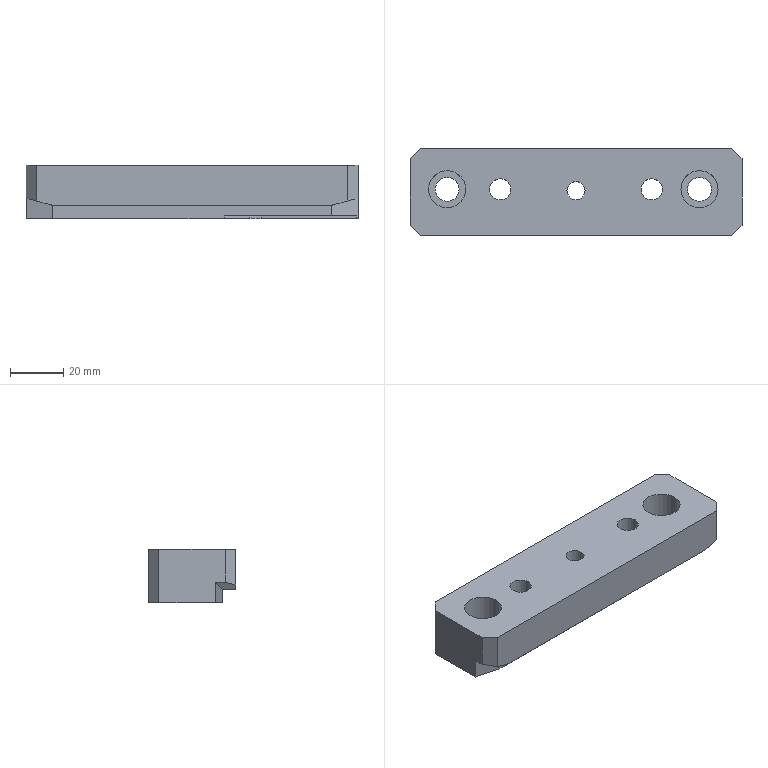Part | NX | features 20 2 | 1 solid | 30 faces | box 125 x 33 x 20 mm | volume 71217 mm3 | plane 21 | cylinder 9 | commonest cylinder face diameters 8.001 x2 9 x2 14 x2 20 x2 6.8 x1
STEP:
#1=CARTESIAN_POINT('',(1124.402,434.5,-3.5));
#2=VERTEX_POINT('',#1);
#3=CARTESIAN_POINT('',(1121.002,434.5,-3.5));
#4=DIRECTION('',(0.,0.,1.));
#5=DIRECTION('',(1.,0.,0.));
#6=AXIS2_PLACEMENT_3D('',#3,#4,#5);
#7=CIRCLE('',#6,3.4);
#8=EDGE_CURVE('',#2,#2,#7,.T.);
#9=ORIENTED_EDGE('',*,*,#8,.T.);
#10=EDGE_LOOP('',(#9));
#11=FACE_BOUND('',#10,.T.);
#12=CARTESIAN_POINT('',(1068.501,422.5,-3.5));
#13=VERTEX_POINT('',#12);
#14=CARTESIAN_POINT('',(1058.502,425.179,-3.5));
#15=VERTEX_POINT('',#14);
#16=CARTESIAN_POINT('',(1068.501,422.5,-3.5));
#17=DIRECTION('',(-0.9659,0.2588,0.));
#18=VECTOR('',#17,1000.);
#19=LINE('',#16,#18);
#20=EDGE_CURVE('',#13,#15,#19,.T.);
#21=ORIENTED_EDGE('',*,*,#20,.T.);
#22=CARTESIAN_POINT('',(1058.502,446.5,-3.5));
#23=VERTEX_POINT('',#22);
#24=CARTESIAN_POINT('',(1058.502,417.5,-3.5));
#25=DIRECTION('',(0.,1.,0.));
#26=VECTOR('',#25,1000.);
#27=LINE('',#24,#26);
#28=EDGE_CURVE('',#15,#23,#27,.T.);
#29=ORIENTED_EDGE('',*,*,#28,.T.);
#30=CARTESIAN_POINT('',(1062.502,450.5,-3.5));
#31=VERTEX_POINT('',#30);
#32=CARTESIAN_POINT('',(1062.502,450.5,-3.5));
#33=DIRECTION('',(-0.7071,-0.7071,0.));
#34=VECTOR('',#33,1000.);
#35=LINE('',#32,#34);
#36=EDGE_CURVE('',#31,#23,#35,.T.);
#37=ORIENTED_EDGE('',*,*,#36,.F.);
#38=CARTESIAN_POINT('',(1179.502,450.5,-3.5));
#39=VERTEX_POINT('',#38);
#40=CARTESIAN_POINT('',(1176.502,450.5,-3.5));
#41=DIRECTION('',(1.,0.,0.));
#42=VECTOR('',#41,1000.);
#43=LINE('',#40,#42);
#44=EDGE_CURVE('',#31,#39,#43,.T.);
#45=ORIENTED_EDGE('',*,*,#44,.T.);
#46=CARTESIAN_POINT('',(1183.502,446.5,-3.5));
#47=VERTEX_POINT('',#46);
#48=CARTESIAN_POINT('',(1183.502,446.5,-3.5));
#49=DIRECTION('',(-0.7071,0.7071,0.));
#50=VECTOR('',#49,1000.);
#51=LINE('',#48,#50);
#52=EDGE_CURVE('',#47,#39,#51,.T.);
#53=ORIENTED_EDGE('',*,*,#52,.F.);
#54=CARTESIAN_POINT('',(1183.502,427.984,-3.5));
#55=VERTEX_POINT('',#54);
#56=CARTESIAN_POINT('',(1183.502,450.5,-3.5));
#57=DIRECTION('',(0.,-1.,0.));
#58=VECTOR('',#57,1000.);
#59=LINE('',#56,#58);
#60=EDGE_CURVE('',#47,#55,#59,.T.);
#61=ORIENTED_EDGE('',*,*,#60,.T.);
#62=CARTESIAN_POINT('',(1182.929,428.,-3.5));
#63=VERTEX_POINT('',#62);
#64=CARTESIAN_POINT('',(1182.929,418.,-3.5));
#65=DIRECTION('',(0.,0.,-1.));
#66=DIRECTION('',(1.,0.,0.));
#67=AXIS2_PLACEMENT_3D('',#64,#65,#66);
#68=CIRCLE('',#67,10.);
#69=EDGE_CURVE('',#63,#55,#68,.T.);
#70=ORIENTED_EDGE('',*,*,#69,.F.);
#71=CARTESIAN_POINT('',(1147.07,428.,-3.5));
#72=VERTEX_POINT('',#71);
#73=CARTESIAN_POINT('',(1066.502,428.,-3.5));
#74=DIRECTION('',(-1.,0.,0.));
#75=VECTOR('',#74,1000.);
#76=LINE('',#73,#75);
#77=EDGE_CURVE('',#63,#72,#76,.T.);
#78=ORIENTED_EDGE('',*,*,#77,.T.);
#79=CARTESIAN_POINT('',(1142.83,427.057,-3.5));
#80=VERTEX_POINT('',#79);
#81=CARTESIAN_POINT('',(1147.07,418.,-3.5));
#82=DIRECTION('',(0.,0.,1.));
#83=DIRECTION('',(1.,0.,0.));
#84=AXIS2_PLACEMENT_3D('',#81,#82,#83);
#85=CIRCLE('',#84,10.);
#86=EDGE_CURVE('',#72,#80,#85,.T.);
#87=ORIENTED_EDGE('',*,*,#86,.T.);
#88=CARTESIAN_POINT('',(1133.095,422.5,-3.5));
#89=VERTEX_POINT('',#88);
#90=CARTESIAN_POINT('',(1089.222,401.964,-3.5));
#91=DIRECTION('',(0.9057,0.4239,0.));
#92=VECTOR('',#91,1000.);
#93=LINE('',#90,#92);
#94=EDGE_CURVE('',#89,#80,#93,.T.);
#95=ORIENTED_EDGE('',*,*,#94,.F.);
#96=CARTESIAN_POINT('',(1154.501,422.5,-3.5));
#97=DIRECTION('',(-1.,0.,0.));
#98=VECTOR('',#97,1000.);
#99=LINE('',#96,#98);
#100=EDGE_CURVE('',#89,#13,#99,.T.);
#101=ORIENTED_EDGE('',*,*,#100,.T.);
#102=EDGE_LOOP('',(#21,#29,#37,#45,#53,#61,#70,#78,#87,#95,#101));
#103=FACE_BOUND('',#102,.T.);
#104=CARTESIAN_POINT('',(1077.002,435.,-3.5));
#105=VERTEX_POINT('',#104);
#106=CARTESIAN_POINT('',(1072.502,435.,-3.5));
#107=DIRECTION('',(0.,0.,1.));
#108=DIRECTION('',(1.,0.,0.));
#109=AXIS2_PLACEMENT_3D('',#106,#107,#108);
#110=CIRCLE('',#109,4.5);
#111=EDGE_CURVE('',#105,#105,#110,.T.);
#112=ORIENTED_EDGE('',*,*,#111,.T.);
#113=EDGE_LOOP('',(#112));
#114=FACE_BOUND('',#113,.T.);
#115=CARTESIAN_POINT('',(1172.002,435.,-3.5));
#116=VERTEX_POINT('',#115);
#117=CARTESIAN_POINT('',(1167.502,435.,-3.5));
#118=DIRECTION('',(0.,0.,-1.));
#119=DIRECTION('',(1.,0.,0.));
#120=AXIS2_PLACEMENT_3D('',#117,#118,#119);
#121=CIRCLE('',#120,4.5);
#122=EDGE_CURVE('',#116,#116,#121,.T.);
#123=ORIENTED_EDGE('',*,*,#122,.F.);
#124=EDGE_LOOP('',(#123));
#125=FACE_BOUND('',#124,.T.);
#126=CARTESIAN_POINT('',(1096.503,435.,-3.5));
#127=VERTEX_POINT('',#126);
#128=CARTESIAN_POINT('',(1092.502,435.,-3.5));
#129=DIRECTION('',(0.,0.,1.));
#130=DIRECTION('',(1.,0.,0.));
#131=AXIS2_PLACEMENT_3D('',#128,#129,#130);
#132=CIRCLE('',#131,4.);
#133=EDGE_CURVE('',#127,#127,#132,.T.);
#134=ORIENTED_EDGE('',*,*,#133,.T.);
#135=EDGE_LOOP('',(#134));
#136=FACE_BOUND('',#135,.T.);
#137=CARTESIAN_POINT('',(1153.503,435.,-3.5));
#138=VERTEX_POINT('',#137);
#139=CARTESIAN_POINT('',(1149.502,435.,-3.5));
#140=DIRECTION('',(0.,0.,-1.));
#141=DIRECTION('',(1.,0.,0.));
#142=AXIS2_PLACEMENT_3D('',#139,#140,#141);
#143=CIRCLE('',#142,4.);
#144=EDGE_CURVE('',#138,#138,#143,.T.);
#145=ORIENTED_EDGE('',*,*,#144,.F.);
#146=EDGE_LOOP('',(#145));
#147=FACE_BOUND('',#146,.T.);
#148=CARTESIAN_POINT('',(1246.502,450.5,-3.5));
#149=DIRECTION('',(0.,0.,1.));
#150=DIRECTION('',(-1.,0.,0.));
#151=AXIS2_PLACEMENT_3D('',#148,#149,#150);
#152=PLANE('',#151);
#153=ADVANCED_FACE('',(#11,#103,#114,#125,#136,#147),#152,.F.);
#154=CARTESIAN_POINT('',(1153.503,435.,16.5));
#155=VERTEX_POINT('',#154);
#156=CARTESIAN_POINT('',(1149.502,435.,16.5));
#157=DIRECTION('',(0.,0.,1.));
#158=DIRECTION('',(1.,0.,0.));
#159=AXIS2_PLACEMENT_3D('',#156,#157,#158);
#160=CIRCLE('',#159,4.);
#161=EDGE_CURVE('',#155,#155,#160,.T.);
#162=ORIENTED_EDGE('',*,*,#161,.F.);
#163=EDGE_LOOP('',(#162));
#164=FACE_BOUND('',#163,.T.);
#165=CARTESIAN_POINT('',(1096.503,435.,16.5));
#166=VERTEX_POINT('',#165);
#167=CARTESIAN_POINT('',(1092.502,435.,16.5));
#168=DIRECTION('',(0.,0.,1.));
#169=DIRECTION('',(1.,0.,0.));
#170=AXIS2_PLACEMENT_3D('',#167,#168,#169);
#171=CIRCLE('',#170,4.);
#172=EDGE_CURVE('',#166,#166,#171,.T.);
#173=ORIENTED_EDGE('',*,*,#172,.F.);
#174=EDGE_LOOP('',(#173));
#175=FACE_BOUND('',#174,.T.);
#176=CARTESIAN_POINT('',(1079.502,435.,16.5));
#177=VERTEX_POINT('',#176);
#178=CARTESIAN_POINT('',(1072.502,435.,16.5));
#179=DIRECTION('',(0.,0.,-1.));
#180=DIRECTION('',(1.,0.,0.));
#181=AXIS2_PLACEMENT_3D('',#178,#179,#180);
#182=CIRCLE('',#181,7.);
#183=EDGE_CURVE('',#177,#177,#182,.T.);
#184=ORIENTED_EDGE('',*,*,#183,.T.);
#185=EDGE_LOOP('',(#184));
#186=FACE_BOUND('',#185,.T.);
#187=CARTESIAN_POINT('',(1183.502,446.5,16.5));
#188=VERTEX_POINT('',#187);
#189=CARTESIAN_POINT('',(1183.502,421.5,16.5));
#190=VERTEX_POINT('',#189);
#191=CARTESIAN_POINT('',(1183.502,450.5,16.5));
#192=DIRECTION('',(0.,-1.,0.));
#193=VECTOR('',#192,1000.);
#194=LINE('',#191,#193);
#195=EDGE_CURVE('',#188,#190,#194,.T.);
#196=ORIENTED_EDGE('',*,*,#195,.F.);
#197=CARTESIAN_POINT('',(1179.502,450.5,16.5));
#198=VERTEX_POINT('',#197);
#199=CARTESIAN_POINT('',(1183.502,446.5,16.5));
#200=DIRECTION('',(0.7071,-0.7071,0.));
#201=VECTOR('',#200,1000.);
#202=LINE('',#199,#201);
#203=EDGE_CURVE('',#198,#188,#202,.T.);
#204=ORIENTED_EDGE('',*,*,#203,.F.);
#205=CARTESIAN_POINT('',(1062.502,450.5,16.5));
#206=VERTEX_POINT('',#205);
#207=CARTESIAN_POINT('',(1136.502,450.5,16.5));
#208=DIRECTION('',(1.,0.,0.));
#209=VECTOR('',#208,1000.);
#210=LINE('',#207,#209);
#211=EDGE_CURVE('',#206,#198,#210,.T.);
#212=ORIENTED_EDGE('',*,*,#211,.F.);
#213=CARTESIAN_POINT('',(1058.502,446.5,16.5));
#214=VERTEX_POINT('',#213);
#215=CARTESIAN_POINT('',(1062.502,450.5,16.5));
#216=DIRECTION('',(0.7071,0.7071,0.));
#217=VECTOR('',#216,1000.);
#218=LINE('',#215,#217);
#219=EDGE_CURVE('',#214,#206,#218,.T.);
#220=ORIENTED_EDGE('',*,*,#219,.F.);
#221=CARTESIAN_POINT('',(1058.502,421.5,16.5));
#222=VERTEX_POINT('',#221);
#223=CARTESIAN_POINT('',(1058.502,417.5,16.5));
#224=DIRECTION('',(0.,1.,0.));
#225=VECTOR('',#224,1000.);
#226=LINE('',#223,#225);
#227=EDGE_CURVE('',#222,#214,#226,.T.);
#228=ORIENTED_EDGE('',*,*,#227,.F.);
#229=CARTESIAN_POINT('',(1062.502,417.5,16.5));
#230=VERTEX_POINT('',#229);
#231=CARTESIAN_POINT('',(1058.502,421.5,16.5));
#232=DIRECTION('',(-0.7071,0.7071,0.));
#233=VECTOR('',#232,1000.);
#234=LINE('',#231,#233);
#235=EDGE_CURVE('',#230,#222,#234,.T.);
#236=ORIENTED_EDGE('',*,*,#235,.F.);
#237=CARTESIAN_POINT('',(1179.502,417.5,16.5));
#238=VERTEX_POINT('',#237);
#239=CARTESIAN_POINT('',(1216.502,417.5,16.5));
#240=DIRECTION('',(-1.,0.,0.));
#241=VECTOR('',#240,1000.);
#242=LINE('',#239,#241);
#243=EDGE_CURVE('',#238,#230,#242,.T.);
#244=ORIENTED_EDGE('',*,*,#243,.F.);
#245=CARTESIAN_POINT('',(1179.502,417.5,16.5));
#246=DIRECTION('',(-0.7071,-0.7071,0.));
#247=VECTOR('',#246,1000.);
#248=LINE('',#245,#247);
#249=EDGE_CURVE('',#190,#238,#248,.T.);
#250=ORIENTED_EDGE('',*,*,#249,.F.);
#251=EDGE_LOOP('',(#196,#204,#212,#220,#228,#236,#244,#250));
#252=FACE_BOUND('',#251,.T.);
#253=CARTESIAN_POINT('',(1174.502,435.,16.5));
#254=VERTEX_POINT('',#253);
#255=CARTESIAN_POINT('',(1167.502,435.,16.5));
#256=DIRECTION('',(0.,0.,-1.));
#257=DIRECTION('',(1.,0.,0.));
#258=AXIS2_PLACEMENT_3D('',#255,#256,#257);
#259=CIRCLE('',#258,7.);
#260=EDGE_CURVE('',#254,#254,#259,.T.);
#261=ORIENTED_EDGE('',*,*,#260,.T.);
#262=EDGE_LOOP('',(#261));
#263=FACE_BOUND('',#262,.T.);
#264=CARTESIAN_POINT('',(1124.402,434.5,16.5));
#265=VERTEX_POINT('',#264);
#266=CARTESIAN_POINT('',(1121.002,434.5,16.5));
#267=DIRECTION('',(0.,0.,1.));
#268=DIRECTION('',(1.,0.,0.));
#269=AXIS2_PLACEMENT_3D('',#266,#267,#268);
#270=CIRCLE('',#269,3.4);
#271=EDGE_CURVE('',#265,#265,#270,.T.);
#272=ORIENTED_EDGE('',*,*,#271,.F.);
#273=EDGE_LOOP('',(#272));
#274=FACE_BOUND('',#273,.T.);
#275=CARTESIAN_POINT('',(1216.502,450.5,16.5));
#276=DIRECTION('',(0.,0.,1.));
#277=DIRECTION('',(-1.,0.,0.));
#278=AXIS2_PLACEMENT_3D('',#275,#276,#277);
#279=PLANE('',#278);
#280=ADVANCED_FACE('',(#164,#175,#186,#252,#263,#274),#279,.T.);
#281=CARTESIAN_POINT('',(1142.83,427.057,-2.5));
#282=VERTEX_POINT('',#281);
#283=CARTESIAN_POINT('',(1147.07,428.,-2.5));
#284=VERTEX_POINT('',#283);
#285=CARTESIAN_POINT('',(1147.07,418.,-2.5));
#286=DIRECTION('',(0.,0.,-1.));
#287=DIRECTION('',(1.,0.,0.));
#288=AXIS2_PLACEMENT_3D('',#285,#286,#287);
#289=CIRCLE('',#288,10.);
#290=EDGE_CURVE('',#282,#284,#289,.T.);
#291=ORIENTED_EDGE('',*,*,#290,.F.);
#292=CARTESIAN_POINT('',(1142.83,427.057,-43.5));
#293=DIRECTION('',(0.,0.,-1.));
#294=VECTOR('',#293,1000.);
#295=LINE('',#292,#294);
#296=EDGE_CURVE('',#282,#80,#295,.T.);
#297=ORIENTED_EDGE('',*,*,#296,.T.);
#298=ORIENTED_EDGE('',*,*,#86,.F.);
#299=CARTESIAN_POINT('',(1147.07,428.,-43.5));
#300=DIRECTION('',(0.,0.,-1.));
#301=VECTOR('',#300,1000.);
#302=LINE('',#299,#301);
#303=EDGE_CURVE('',#284,#72,#302,.T.);
#304=ORIENTED_EDGE('',*,*,#303,.F.);
#305=EDGE_LOOP('',(#291,#297,#298,#304));
#306=FACE_BOUND('',#305,.T.);
#307=CARTESIAN_POINT('',(1147.07,418.,-43.5));
#308=DIRECTION('',(0.,0.,1.));
#309=DIRECTION('',(-1.,0.,0.));
#310=AXIS2_PLACEMENT_3D('',#307,#308,#309);
#311=CYLINDRICAL_SURFACE('',#310,10.);
#312=ADVANCED_FACE('',(#306),#311,.F.);
#313=CARTESIAN_POINT('',(1133.095,422.5,-2.5));
#314=VERTEX_POINT('',#313);
#315=CARTESIAN_POINT('',(1091.314,402.943,-2.5));
#316=DIRECTION('',(-0.9057,-0.4239,0.));
#317=VECTOR('',#316,1000.);
#318=LINE('',#315,#317);
#319=EDGE_CURVE('',#282,#314,#318,.T.);
#320=ORIENTED_EDGE('',*,*,#319,.T.);
#321=CARTESIAN_POINT('',(1133.095,422.5,3.5));
#322=DIRECTION('',(0.,0.,-1.));
#323=VECTOR('',#322,1000.);
#324=LINE('',#321,#323);
#325=EDGE_CURVE('',#314,#89,#324,.T.);
#326=ORIENTED_EDGE('',*,*,#325,.T.);
#327=ORIENTED_EDGE('',*,*,#94,.T.);
#328=ORIENTED_EDGE('',*,*,#296,.F.);
#329=EDGE_LOOP('',(#320,#326,#327,#328));
#330=FACE_BOUND('',#329,.T.);
#331=CARTESIAN_POINT('',(1091.314,402.943,-43.5));
#332=DIRECTION('',(-0.4239,0.9057,0.));
#333=DIRECTION('',(-0.9057,-0.4239,0.));
#334=AXIS2_PLACEMENT_3D('',#331,#332,#333);
#335=PLANE('',#334);
#336=ADVANCED_FACE('',(#330),#335,.F.);
#337=CARTESIAN_POINT('',(1183.502,427.984,-2.5));
#338=VERTEX_POINT('',#337);
#339=CARTESIAN_POINT('',(1182.929,428.,-2.5));
#340=VERTEX_POINT('',#339);
#341=CARTESIAN_POINT('',(1182.929,418.,-2.5));
#342=DIRECTION('',(0.,0.,1.));
#343=DIRECTION('',(1.,0.,0.));
#344=AXIS2_PLACEMENT_3D('',#341,#342,#343);
#345=CIRCLE('',#344,10.);
#346=EDGE_CURVE('',#338,#340,#345,.T.);
#347=ORIENTED_EDGE('',*,*,#346,.T.);
#348=CARTESIAN_POINT('',(1182.929,428.,-43.5));
#349=DIRECTION('',(0.,0.,-1.));
#350=VECTOR('',#349,1000.);
#351=LINE('',#348,#350);
#352=EDGE_CURVE('',#340,#63,#351,.T.);
#353=ORIENTED_EDGE('',*,*,#352,.T.);
#354=ORIENTED_EDGE('',*,*,#69,.T.);
#355=CARTESIAN_POINT('',(1183.502,427.984,-43.5));
#356=DIRECTION('',(0.,0.,1.));
#357=VECTOR('',#356,1000.);
#358=LINE('',#355,#357);
#359=EDGE_CURVE('',#55,#338,#358,.T.);
#360=ORIENTED_EDGE('',*,*,#359,.T.);
#361=EDGE_LOOP('',(#347,#353,#354,#360));
#362=FACE_BOUND('',#361,.T.);
#363=CARTESIAN_POINT('',(1182.929,418.,-43.5));
#364=DIRECTION('',(0.,0.,1.));
#365=DIRECTION('',(-1.,0.,0.));
#366=AXIS2_PLACEMENT_3D('',#363,#364,#365);
#367=CYLINDRICAL_SURFACE('',#366,10.);
#368=ADVANCED_FACE('',(#362),#367,.F.);
#369=CARTESIAN_POINT('',(1163.002,435.,6.5));
#370=VERTEX_POINT('',#369);
#371=CARTESIAN_POINT('',(1167.502,435.,6.5));
#372=DIRECTION('',(0.,0.,1.));
#373=DIRECTION('',(-1.,0.,0.));
#374=AXIS2_PLACEMENT_3D('',#371,#372,#373);
#375=CIRCLE('',#374,4.5);
#376=EDGE_CURVE('',#370,#370,#375,.T.);
#377=ORIENTED_EDGE('',*,*,#376,.F.);
#378=EDGE_LOOP('',(#377));
#379=FACE_BOUND('',#378,.T.);
#380=CARTESIAN_POINT('',(1160.502,435.,6.5));
#381=VERTEX_POINT('',#380);
#382=CARTESIAN_POINT('',(1167.502,435.,6.5));
#383=DIRECTION('',(0.,0.,-1.));
#384=DIRECTION('',(-1.,0.,0.));
#385=AXIS2_PLACEMENT_3D('',#382,#383,#384);
#386=CIRCLE('',#385,7.);
#387=EDGE_CURVE('',#381,#381,#386,.T.);
#388=ORIENTED_EDGE('',*,*,#387,.F.);
#389=EDGE_LOOP('',(#388));
#390=FACE_BOUND('',#389,.T.);
#391=CARTESIAN_POINT('',(1167.502,432.5,6.5));
#392=DIRECTION('',(0.,0.,-1.));
#393=DIRECTION('',(1.,0.,0.));
#394=AXIS2_PLACEMENT_3D('',#391,#392,#393);
#395=PLANE('',#394);
#396=ADVANCED_FACE('',(#379,#390),#395,.F.);
#397=CARTESIAN_POINT('',(1068.002,435.,6.5));
#398=VERTEX_POINT('',#397);
#399=CARTESIAN_POINT('',(1072.502,435.,6.5));
#400=DIRECTION('',(0.,0.,1.));
#401=DIRECTION('',(-1.,0.,0.));
#402=AXIS2_PLACEMENT_3D('',#399,#400,#401);
#403=CIRCLE('',#402,4.5);
#404=EDGE_CURVE('',#398,#398,#403,.T.);
#405=ORIENTED_EDGE('',*,*,#404,.F.);
#406=EDGE_LOOP('',(#405));
#407=FACE_BOUND('',#406,.T.);
#408=CARTESIAN_POINT('',(1065.502,435.,6.5));
#409=VERTEX_POINT('',#408);
#410=CARTESIAN_POINT('',(1072.502,435.,6.5));
#411=DIRECTION('',(0.,0.,-1.));
#412=DIRECTION('',(-1.,0.,0.));
#413=AXIS2_PLACEMENT_3D('',#410,#411,#412);
#414=CIRCLE('',#413,7.);
#415=EDGE_CURVE('',#409,#409,#414,.T.);
#416=ORIENTED_EDGE('',*,*,#415,.F.);
#417=EDGE_LOOP('',(#416));
#418=FACE_BOUND('',#417,.T.);
#419=CARTESIAN_POINT('',(1072.502,432.5,6.5));
#420=DIRECTION('',(0.,0.,-1.));
#421=DIRECTION('',(-1.,0.,0.));
#422=AXIS2_PLACEMENT_3D('',#419,#420,#421);
#423=PLANE('',#422);
#424=ADVANCED_FACE('',(#407,#418),#423,.F.);
#425=ORIENTED_EDGE('',*,*,#260,.F.);
#426=EDGE_LOOP('',(#425));
#427=FACE_BOUND('',#426,.T.);
#428=ORIENTED_EDGE('',*,*,#387,.T.);
#429=EDGE_LOOP('',(#428));
#430=FACE_BOUND('',#429,.T.);
#431=CARTESIAN_POINT('',(1167.502,435.,42.5));
#432=DIRECTION('',(0.,0.,-1.));
#433=DIRECTION('',(1.,0.,0.));
#434=AXIS2_PLACEMENT_3D('',#431,#432,#433);
#435=CYLINDRICAL_SURFACE('',#434,7.);
#436=ADVANCED_FACE('',(#427,#430),#435,.F.);
#437=ORIENTED_EDGE('',*,*,#415,.T.);
#438=EDGE_LOOP('',(#437));
#439=FACE_BOUND('',#438,.T.);
#440=ORIENTED_EDGE('',*,*,#183,.F.);
#441=EDGE_LOOP('',(#440));
#442=FACE_BOUND('',#441,.T.);
#443=CARTESIAN_POINT('',(1072.502,435.,42.5));
#444=DIRECTION('',(0.,0.,-1.));
#445=DIRECTION('',(-1.,0.,0.));
#446=AXIS2_PLACEMENT_3D('',#443,#444,#445);
#447=CYLINDRICAL_SURFACE('',#446,7.);
#448=ADVANCED_FACE('',(#439,#442),#447,.F.);
#449=ORIENTED_EDGE('',*,*,#60,.F.);
#450=CARTESIAN_POINT('',(1183.502,446.5,11.5));
#451=DIRECTION('',(0.,0.,-1.));
#452=VECTOR('',#451,1000.);
#453=LINE('',#450,#452);
#454=EDGE_CURVE('',#188,#47,#453,.T.);
#455=ORIENTED_EDGE('',*,*,#454,.F.);
#456=ORIENTED_EDGE('',*,*,#195,.T.);
#457=CARTESIAN_POINT('',(1183.502,421.5,4.179));
#458=VERTEX_POINT('',#457);
#459=CARTESIAN_POINT('',(1183.502,421.5,11.5));
#460=DIRECTION('',(0.,0.,1.));
#461=VECTOR('',#460,1000.);
#462=LINE('',#459,#461);
#463=EDGE_CURVE('',#458,#190,#462,.T.);
#464=ORIENTED_EDGE('',*,*,#463,.F.);
#465=CARTESIAN_POINT('',(1183.502,425.18,4.179));
#466=VERTEX_POINT('',#465);
#467=CARTESIAN_POINT('',(1183.502,417.5,4.179));
#468=DIRECTION('',(0.,-1.,0.));
#469=VECTOR('',#468,1000.);
#470=LINE('',#467,#469);
#471=EDGE_CURVE('',#466,#458,#470,.T.);
#472=ORIENTED_EDGE('',*,*,#471,.F.);
#473=CARTESIAN_POINT('',(1183.502,425.18,-2.5));
#474=VERTEX_POINT('',#473);
#475=CARTESIAN_POINT('',(1183.502,425.18,3.5));
#476=DIRECTION('',(0.,0.,-1.));
#477=VECTOR('',#476,1000.);
#478=LINE('',#475,#477);
#479=EDGE_CURVE('',#466,#474,#478,.T.);
#480=ORIENTED_EDGE('',*,*,#479,.T.);
#481=CARTESIAN_POINT('',(1183.502,450.5,-2.5));
#482=DIRECTION('',(0.,-1.,0.));
#483=VECTOR('',#482,1000.);
#484=LINE('',#481,#483);
#485=EDGE_CURVE('',#338,#474,#484,.T.);
#486=ORIENTED_EDGE('',*,*,#485,.F.);
#487=ORIENTED_EDGE('',*,*,#359,.F.);
#488=EDGE_LOOP('',(#449,#455,#456,#464,#472,#480,#486,#487));
#489=FACE_BOUND('',#488,.T.);
#490=CARTESIAN_POINT('',(1183.502,450.5,11.5));
#491=DIRECTION('',(-1.,0.,0.));
#492=DIRECTION('',(0.,0.,-1.));
#493=AXIS2_PLACEMENT_3D('',#490,#491,#492);
#494=PLANE('',#493);
#495=ADVANCED_FACE('',(#489),#494,.F.);
#496=ORIENTED_EDGE('',*,*,#376,.T.);
#497=EDGE_LOOP('',(#496));
#498=FACE_BOUND('',#497,.T.);
#499=ORIENTED_EDGE('',*,*,#122,.T.);
#500=EDGE_LOOP('',(#499));
#501=FACE_BOUND('',#500,.T.);
#502=CARTESIAN_POINT('',(1167.502,435.,42.5));
#503=DIRECTION('',(0.,0.,-1.));
#504=DIRECTION('',(1.,0.,0.));
#505=AXIS2_PLACEMENT_3D('',#502,#503,#504);
#506=CYLINDRICAL_SURFACE('',#505,4.5);
#507=ADVANCED_FACE('',(#498,#501),#506,.F.);
#508=ORIENTED_EDGE('',*,*,#243,.T.);
#509=CARTESIAN_POINT('',(1062.502,417.5,3.108));
#510=VERTEX_POINT('',#509);
#511=CARTESIAN_POINT('',(1062.502,417.5,11.5));
#512=DIRECTION('',(0.,0.,1.));
#513=VECTOR('',#512,1000.);
#514=LINE('',#511,#513);
#515=EDGE_CURVE('',#510,#230,#514,.T.);
#516=ORIENTED_EDGE('',*,*,#515,.F.);
#517=CARTESIAN_POINT('',(1068.502,417.5,1.5));
#518=VERTEX_POINT('',#517);
#519=CARTESIAN_POINT('',(1068.502,417.5,1.5));
#520=DIRECTION('',(-0.9659,0.,0.2588));
#521=VECTOR('',#520,1000.);
#522=LINE('',#519,#521);
#523=EDGE_CURVE('',#518,#510,#522,.T.);
#524=ORIENTED_EDGE('',*,*,#523,.F.);
#525=CARTESIAN_POINT('',(1173.502,417.5,1.5));
#526=VERTEX_POINT('',#525);
#527=CARTESIAN_POINT('',(1194.502,417.5,1.5));
#528=DIRECTION('',(1.,0.,0.));
#529=VECTOR('',#528,1000.);
#530=LINE('',#527,#529);
#531=EDGE_CURVE('',#518,#526,#530,.T.);
#532=ORIENTED_EDGE('',*,*,#531,.T.);
#533=CARTESIAN_POINT('',(1179.502,417.5,3.108));
#534=VERTEX_POINT('',#533);
#535=CARTESIAN_POINT('',(1173.502,417.5,1.5));
#536=DIRECTION('',(-0.9659,0.,-0.2588));
#537=VECTOR('',#536,1000.);
#538=LINE('',#535,#537);
#539=EDGE_CURVE('',#534,#526,#538,.T.);
#540=ORIENTED_EDGE('',*,*,#539,.F.);
#541=CARTESIAN_POINT('',(1179.502,417.5,11.5));
#542=DIRECTION('',(0.,0.,-1.));
#543=VECTOR('',#542,1000.);
#544=LINE('',#541,#543);
#545=EDGE_CURVE('',#238,#534,#544,.T.);
#546=ORIENTED_EDGE('',*,*,#545,.F.);
#547=EDGE_LOOP('',(#508,#516,#524,#532,#540,#546));
#548=FACE_BOUND('',#547,.T.);
#549=CARTESIAN_POINT('',(1216.502,417.5,11.5));
#550=DIRECTION('',(0.,1.,0.));
#551=DIRECTION('',(0.,0.,1.));
#552=AXIS2_PLACEMENT_3D('',#549,#550,#551);
#553=PLANE('',#552);
#554=ADVANCED_FACE('',(#548),#553,.F.);
#555=ORIENTED_EDGE('',*,*,#235,.T.);
#556=CARTESIAN_POINT('',(1058.502,421.5,4.179));
#557=VERTEX_POINT('',#556);
#558=CARTESIAN_POINT('',(1058.502,421.5,11.5));
#559=DIRECTION('',(0.,0.,-1.));
#560=VECTOR('',#559,1000.);
#561=LINE('',#558,#560);
#562=EDGE_CURVE('',#222,#557,#561,.T.);
#563=ORIENTED_EDGE('',*,*,#562,.T.);
#564=CARTESIAN_POINT('',(1075.554,404.449,-0.3894));
#565=DIRECTION('',(0.6947,-0.6947,-0.1862));
#566=VECTOR('',#565,1000.);
#567=LINE('',#564,#566);
#568=EDGE_CURVE('',#557,#510,#567,.T.);
#569=ORIENTED_EDGE('',*,*,#568,.T.);
#570=ORIENTED_EDGE('',*,*,#515,.T.);
#571=EDGE_LOOP('',(#555,#563,#569,#570));
#572=FACE_BOUND('',#571,.T.);
#573=CARTESIAN_POINT('',(1058.502,421.5,11.5));
#574=DIRECTION('',(0.7071,0.7071,0.));
#575=DIRECTION('',(0.,0.,-1.));
#576=AXIS2_PLACEMENT_3D('',#573,#574,#575);
#577=PLANE('',#576);
#578=ADVANCED_FACE('',(#572),#577,.F.);
#579=ORIENTED_EDGE('',*,*,#111,.F.);
#580=EDGE_LOOP('',(#579));
#581=FACE_BOUND('',#580,.T.);
#582=ORIENTED_EDGE('',*,*,#404,.T.);
#583=EDGE_LOOP('',(#582));
#584=FACE_BOUND('',#583,.T.);
#585=CARTESIAN_POINT('',(1072.502,435.,42.5));
#586=DIRECTION('',(0.,0.,-1.));
#587=DIRECTION('',(-1.,0.,0.));
#588=AXIS2_PLACEMENT_3D('',#585,#586,#587);
#589=CYLINDRICAL_SURFACE('',#588,4.5);
#590=ADVANCED_FACE('',(#581,#584),#589,.F.);
#591=ORIENTED_EDGE('',*,*,#227,.T.);
#592=CARTESIAN_POINT('',(1058.502,446.5,11.5));
#593=DIRECTION('',(0.,0.,1.));
#594=VECTOR('',#593,1000.);
#595=LINE('',#592,#594);
#596=EDGE_CURVE('',#23,#214,#595,.T.);
#597=ORIENTED_EDGE('',*,*,#596,.F.);
#598=ORIENTED_EDGE('',*,*,#28,.F.);
#599=CARTESIAN_POINT('',(1058.502,425.179,4.179));
#600=VERTEX_POINT('',#599);
#601=CARTESIAN_POINT('',(1058.502,425.179,3.5));
#602=DIRECTION('',(0.,0.,-1.));
#603=VECTOR('',#602,1000.);
#604=LINE('',#601,#603);
#605=EDGE_CURVE('',#600,#15,#604,.T.);
#606=ORIENTED_EDGE('',*,*,#605,.F.);
#607=CARTESIAN_POINT('',(1058.502,425.179,4.179));
#608=DIRECTION('',(0.,1.,0.));
#609=VECTOR('',#608,1000.);
#610=LINE('',#607,#609);
#611=EDGE_CURVE('',#557,#600,#610,.T.);
#612=ORIENTED_EDGE('',*,*,#611,.F.);
#613=ORIENTED_EDGE('',*,*,#562,.F.);
#614=EDGE_LOOP('',(#591,#597,#598,#606,#612,#613));
#615=FACE_BOUND('',#614,.T.);
#616=CARTESIAN_POINT('',(1058.502,417.5,11.5));
#617=DIRECTION('',(1.,0.,0.));
#618=DIRECTION('',(0.,0.,1.));
#619=AXIS2_PLACEMENT_3D('',#616,#617,#618);
#620=PLANE('',#619);
#621=ADVANCED_FACE('',(#615),#620,.F.);
#622=ORIENTED_EDGE('',*,*,#611,.T.);
#623=CARTESIAN_POINT('',(1068.501,422.5,1.5));
#624=VERTEX_POINT('',#623);
#625=CARTESIAN_POINT('',(1068.501,422.5,1.5));
#626=DIRECTION('',(0.9351,-0.2506,-0.2506));
#627=VECTOR('',#626,1000.);
#628=LINE('',#625,#627);
#629=EDGE_CURVE('',#600,#624,#628,.T.);
#630=ORIENTED_EDGE('',*,*,#629,.T.);
#631=CARTESIAN_POINT('',(1068.502,422.5,1.5));
#632=VERTEX_POINT('',#631);
#633=CARTESIAN_POINT('',(1068.502,422.5,1.5));
#634=DIRECTION('',(0.9659,0.,-0.2588));
#635=VECTOR('',#634,1000.);
#636=LINE('',#633,#635);
#637=EDGE_CURVE('',#624,#632,#636,.T.);
#638=ORIENTED_EDGE('',*,*,#637,.T.);
#639=CARTESIAN_POINT('',(1068.502,417.5,1.5));
#640=DIRECTION('',(0.,-1.,0.));
#641=VECTOR('',#640,1000.);
#642=LINE('',#639,#641);
#643=EDGE_CURVE('',#632,#518,#642,.T.);
#644=ORIENTED_EDGE('',*,*,#643,.T.);
#645=ORIENTED_EDGE('',*,*,#523,.T.);
#646=ORIENTED_EDGE('',*,*,#568,.F.);
#647=EDGE_LOOP('',(#622,#630,#638,#644,#645,#646));
#648=FACE_BOUND('',#647,.T.);
#649=CARTESIAN_POINT('',(1068.502,396.891,1.5));
#650=DIRECTION('',(-0.2588,0.,-0.9659));
#651=DIRECTION('',(0.9659,0.,-0.2588));
#652=AXIS2_PLACEMENT_3D('',#649,#650,#651);
#653=PLANE('',#652);
#654=ADVANCED_FACE('',(#648),#653,.T.);
#655=ORIENTED_EDGE('',*,*,#20,.F.);
#656=CARTESIAN_POINT('',(1068.501,422.5,3.5));
#657=DIRECTION('',(0.,0.,1.));
#658=VECTOR('',#657,1000.);
#659=LINE('',#656,#658);
#660=EDGE_CURVE('',#13,#624,#659,.T.);
#661=ORIENTED_EDGE('',*,*,#660,.T.);
#662=ORIENTED_EDGE('',*,*,#629,.F.);
#663=ORIENTED_EDGE('',*,*,#605,.T.);
#664=EDGE_LOOP('',(#655,#661,#662,#663));
#665=FACE_BOUND('',#664,.T.);
#666=CARTESIAN_POINT('',(1068.501,422.5,3.5));
#667=DIRECTION('',(0.2588,0.9659,0.));
#668=DIRECTION('',(0.9659,-0.2588,0.));
#669=AXIS2_PLACEMENT_3D('',#666,#667,#668);
#670=PLANE('',#669);
#671=ADVANCED_FACE('',(#665),#670,.F.);
#672=ORIENTED_EDGE('',*,*,#36,.T.);
#673=ORIENTED_EDGE('',*,*,#596,.T.);
#674=ORIENTED_EDGE('',*,*,#219,.T.);
#675=CARTESIAN_POINT('',(1062.502,450.5,11.5));
#676=DIRECTION('',(0.,0.,-1.));
#677=VECTOR('',#676,1000.);
#678=LINE('',#675,#677);
#679=EDGE_CURVE('',#206,#31,#678,.T.);
#680=ORIENTED_EDGE('',*,*,#679,.T.);
#681=EDGE_LOOP('',(#672,#673,#674,#680));
#682=FACE_BOUND('',#681,.T.);
#683=CARTESIAN_POINT('',(1062.502,450.5,11.5));
#684=DIRECTION('',(0.7071,-0.7071,0.));
#685=DIRECTION('',(0.,0.,-1.));
#686=AXIS2_PLACEMENT_3D('',#683,#684,#685);
#687=PLANE('',#686);
#688=ADVANCED_FACE('',(#682),#687,.F.);
#689=ORIENTED_EDGE('',*,*,#52,.T.);
#690=CARTESIAN_POINT('',(1179.502,450.5,11.5));
#691=DIRECTION('',(0.,0.,1.));
#692=VECTOR('',#691,1000.);
#693=LINE('',#690,#692);
#694=EDGE_CURVE('',#39,#198,#693,.T.);
#695=ORIENTED_EDGE('',*,*,#694,.T.);
#696=ORIENTED_EDGE('',*,*,#203,.T.);
#697=ORIENTED_EDGE('',*,*,#454,.T.);
#698=EDGE_LOOP('',(#689,#695,#696,#697));
#699=FACE_BOUND('',#698,.T.);
#700=CARTESIAN_POINT('',(1183.502,446.5,11.5));
#701=DIRECTION('',(-0.7071,-0.7071,0.));
#702=DIRECTION('',(0.,0.,-1.));
#703=AXIS2_PLACEMENT_3D('',#700,#701,#702);
#704=PLANE('',#703);
#705=ADVANCED_FACE('',(#699),#704,.F.);
#706=ORIENTED_EDGE('',*,*,#694,.F.);
#707=ORIENTED_EDGE('',*,*,#44,.F.);
#708=ORIENTED_EDGE('',*,*,#679,.F.);
#709=ORIENTED_EDGE('',*,*,#211,.T.);
#710=EDGE_LOOP('',(#706,#707,#708,#709));
#711=FACE_BOUND('',#710,.T.);
#712=CARTESIAN_POINT('',(1136.502,450.5,11.5));
#713=DIRECTION('',(0.,-1.,0.));
#714=DIRECTION('',(0.,0.,-1.));
#715=AXIS2_PLACEMENT_3D('',#712,#713,#714);
#716=PLANE('',#715);
#717=ADVANCED_FACE('',(#711),#716,.F.);
#718=ORIENTED_EDGE('',*,*,#531,.F.);
#719=ORIENTED_EDGE('',*,*,#643,.F.);
#720=CARTESIAN_POINT('',(1173.501,422.5,1.5));
#721=VERTEX_POINT('',#720);
#722=CARTESIAN_POINT('',(1184.501,422.5,1.5));
#723=DIRECTION('',(1.,0.,0.));
#724=VECTOR('',#723,1000.);
#725=LINE('',#722,#724);
#726=EDGE_CURVE('',#632,#721,#725,.T.);
#727=ORIENTED_EDGE('',*,*,#726,.T.);
#728=CARTESIAN_POINT('',(1173.502,422.5,1.5));
#729=VERTEX_POINT('',#728);
#730=CARTESIAN_POINT('',(1183.502,425.18,1.5));
#731=DIRECTION('',(0.9659,0.2588,0.));
#732=VECTOR('',#731,1000.);
#733=LINE('',#730,#732);
#734=EDGE_CURVE('',#721,#729,#733,.T.);
#735=ORIENTED_EDGE('',*,*,#734,.T.);
#736=CARTESIAN_POINT('',(1173.502,425.18,1.5));
#737=DIRECTION('',(0.,1.,0.));
#738=VECTOR('',#737,1000.);
#739=LINE('',#736,#738);
#740=EDGE_CURVE('',#526,#729,#739,.T.);
#741=ORIENTED_EDGE('',*,*,#740,.F.);
#742=EDGE_LOOP('',(#718,#719,#727,#735,#741));
#743=FACE_BOUND('',#742,.T.);
#744=CARTESIAN_POINT('',(1216.773,396.891,1.5));
#745=DIRECTION('',(0.,0.,-1.));
#746=DIRECTION('',(1.,0.,0.));
#747=AXIS2_PLACEMENT_3D('',#744,#745,#746);
#748=PLANE('',#747);
#749=ADVANCED_FACE('',(#743),#748,.T.);
#750=ORIENTED_EDGE('',*,*,#726,.F.);
#751=ORIENTED_EDGE('',*,*,#637,.F.);
#752=ORIENTED_EDGE('',*,*,#660,.F.);
#753=ORIENTED_EDGE('',*,*,#100,.F.);
#754=ORIENTED_EDGE('',*,*,#325,.F.);
#755=CARTESIAN_POINT('',(1173.501,422.5,-2.5));
#756=VERTEX_POINT('',#755);
#757=CARTESIAN_POINT('',(1116.501,422.5,-2.5));
#758=DIRECTION('',(-1.,0.,0.));
#759=VECTOR('',#758,1000.);
#760=LINE('',#757,#759);
#761=EDGE_CURVE('',#756,#314,#760,.T.);
#762=ORIENTED_EDGE('',*,*,#761,.F.);
#763=CARTESIAN_POINT('',(1173.501,422.5,3.5));
#764=DIRECTION('',(0.,0.,1.));
#765=VECTOR('',#764,1000.);
#766=LINE('',#763,#765);
#767=EDGE_CURVE('',#756,#721,#766,.T.);
#768=ORIENTED_EDGE('',*,*,#767,.T.);
#769=EDGE_LOOP('',(#750,#751,#752,#753,#754,#762,#768));
#770=FACE_BOUND('',#769,.T.);
#771=CARTESIAN_POINT('',(1184.501,422.5,3.5));
#772=DIRECTION('',(0.,1.,0.));
#773=DIRECTION('',(0.,0.,1.));
#774=AXIS2_PLACEMENT_3D('',#771,#772,#773);
#775=PLANE('',#774);
#776=ADVANCED_FACE('',(#770),#775,.F.);
#777=ORIENTED_EDGE('',*,*,#303,.T.);
#778=ORIENTED_EDGE('',*,*,#77,.F.);
#779=ORIENTED_EDGE('',*,*,#352,.F.);
#780=CARTESIAN_POINT('',(1066.502,428.,-2.5));
#781=DIRECTION('',(1.,0.,0.));
#782=VECTOR('',#781,1000.);
#783=LINE('',#780,#782);
#784=EDGE_CURVE('',#284,#340,#783,.T.);
#785=ORIENTED_EDGE('',*,*,#784,.F.);
#786=EDGE_LOOP('',(#777,#778,#779,#785));
#787=FACE_BOUND('',#786,.T.);
#788=CARTESIAN_POINT('',(1147.07,428.,-43.5));
#789=DIRECTION('',(0.,1.,0.));
#790=DIRECTION('',(0.,0.,1.));
#791=AXIS2_PLACEMENT_3D('',#788,#789,#790);
#792=PLANE('',#791);
#793=ADVANCED_FACE('',(#787),#792,.F.);
#794=ORIENTED_EDGE('',*,*,#740,.T.);
#795=CARTESIAN_POINT('',(1182.875,425.012,4.011));
#796=DIRECTION('',(0.9351,0.2506,0.2506));
#797=VECTOR('',#796,1000.);
#798=LINE('',#795,#797);
#799=EDGE_CURVE('',#729,#466,#798,.T.);
#800=ORIENTED_EDGE('',*,*,#799,.T.);
#801=ORIENTED_EDGE('',*,*,#471,.T.);
#802=CARTESIAN_POINT('',(1166.451,404.449,-0.3894));
#803=DIRECTION('',(0.6947,0.6947,0.1862));
#804=VECTOR('',#803,1000.);
#805=LINE('',#802,#804);
#806=EDGE_CURVE('',#534,#458,#805,.T.);
#807=ORIENTED_EDGE('',*,*,#806,.F.);
#808=ORIENTED_EDGE('',*,*,#539,.T.);
#809=EDGE_LOOP('',(#794,#800,#801,#807,#808));
#810=FACE_BOUND('',#809,.T.);
#811=CARTESIAN_POINT('',(1173.502,396.891,1.5));
#812=DIRECTION('',(0.2588,0.,-0.9659));
#813=DIRECTION('',(0.9659,0.,0.2588));
#814=AXIS2_PLACEMENT_3D('',#811,#812,#813);
#815=PLANE('',#814);
#816=ADVANCED_FACE('',(#810),#815,.T.);
#817=ORIENTED_EDGE('',*,*,#249,.T.);
#818=ORIENTED_EDGE('',*,*,#545,.T.);
#819=ORIENTED_EDGE('',*,*,#806,.T.);
#820=ORIENTED_EDGE('',*,*,#463,.T.);
#821=EDGE_LOOP('',(#817,#818,#819,#820));
#822=FACE_BOUND('',#821,.T.);
#823=CARTESIAN_POINT('',(1179.502,417.5,11.5));
#824=DIRECTION('',(-0.7071,0.7071,0.));
#825=DIRECTION('',(0.,0.,-1.));
#826=AXIS2_PLACEMENT_3D('',#823,#824,#825);
#827=PLANE('',#826);
#828=ADVANCED_FACE('',(#822),#827,.F.);
#829=ORIENTED_EDGE('',*,*,#734,.F.);
#830=ORIENTED_EDGE('',*,*,#767,.F.);
#831=CARTESIAN_POINT('',(1183.502,425.18,-2.5));
#832=DIRECTION('',(-0.9659,-0.2588,0.));
#833=VECTOR('',#832,1000.);
#834=LINE('',#831,#833);
#835=EDGE_CURVE('',#474,#756,#834,.T.);
#836=ORIENTED_EDGE('',*,*,#835,.F.);
#837=ORIENTED_EDGE('',*,*,#479,.F.);
#838=ORIENTED_EDGE('',*,*,#799,.F.);
#839=EDGE_LOOP('',(#829,#830,#836,#837,#838));
#840=FACE_BOUND('',#839,.T.);
#841=CARTESIAN_POINT('',(1183.502,425.18,3.5));
#842=DIRECTION('',(-0.2588,0.9659,0.));
#843=DIRECTION('',(0.9659,0.2588,0.));
#844=AXIS2_PLACEMENT_3D('',#841,#842,#843);
#845=PLANE('',#844);
#846=ADVANCED_FACE('',(#840),#845,.F.);
#847=ORIENTED_EDGE('',*,*,#319,.F.);
#848=ORIENTED_EDGE('',*,*,#290,.T.);
#849=ORIENTED_EDGE('',*,*,#784,.T.);
#850=ORIENTED_EDGE('',*,*,#346,.F.);
#851=ORIENTED_EDGE('',*,*,#485,.T.);
#852=ORIENTED_EDGE('',*,*,#835,.T.);
#853=ORIENTED_EDGE('',*,*,#761,.T.);
#854=EDGE_LOOP('',(#847,#848,#849,#850,#851,#852,#853));
#855=FACE_BOUND('',#854,.T.);
#856=CARTESIAN_POINT('',(1066.502,450.5,-2.5));
#857=DIRECTION('',(0.,0.,1.));
#858=DIRECTION('',(-1.,0.,0.));
#859=AXIS2_PLACEMENT_3D('',#856,#857,#858);
#860=PLANE('',#859);
#861=ADVANCED_FACE('',(#855),#860,.F.);
#862=ORIENTED_EDGE('',*,*,#271,.T.);
#863=EDGE_LOOP('',(#862));
#864=FACE_BOUND('',#863,.T.);
#865=ORIENTED_EDGE('',*,*,#8,.F.);
#866=EDGE_LOOP('',(#865));
#867=FACE_BOUND('',#866,.T.);
#868=CARTESIAN_POINT('',(1121.002,434.5,16.5));
#869=DIRECTION('',(0.,0.,-1.));
#870=DIRECTION('',(-1.,0.,0.));
#871=AXIS2_PLACEMENT_3D('',#868,#869,#870);
#872=CYLINDRICAL_SURFACE('',#871,3.4);
#873=ADVANCED_FACE('',(#864,#867),#872,.F.);
#874=ORIENTED_EDGE('',*,*,#172,.T.);
#875=EDGE_LOOP('',(#874));
#876=FACE_BOUND('',#875,.T.);
#877=ORIENTED_EDGE('',*,*,#133,.F.);
#878=EDGE_LOOP('',(#877));
#879=FACE_BOUND('',#878,.T.);
#880=CARTESIAN_POINT('',(1092.502,435.,-3.5));
#881=DIRECTION('',(0.,0.,1.));
#882=DIRECTION('',(-1.,0.,0.));
#883=AXIS2_PLACEMENT_3D('',#880,#881,#882);
#884=CYLINDRICAL_SURFACE('',#883,4.);
#885=ADVANCED_FACE('',(#876,#879),#884,.F.);
#886=ORIENTED_EDGE('',*,*,#161,.T.);
#887=EDGE_LOOP('',(#886));
#888=FACE_BOUND('',#887,.T.);
#889=ORIENTED_EDGE('',*,*,#144,.T.);
#890=EDGE_LOOP('',(#889));
#891=FACE_BOUND('',#890,.T.);
#892=CARTESIAN_POINT('',(1149.502,435.,-3.5));
#893=DIRECTION('',(0.,0.,1.));
#894=DIRECTION('',(1.,0.,0.));
#895=AXIS2_PLACEMENT_3D('',#892,#893,#894);
#896=CYLINDRICAL_SURFACE('',#895,4.);
#897=ADVANCED_FACE('',(#888,#891),#896,.F.);
#898=CLOSED_SHELL('',(#153,#280,#312,#336,#368,#396,#424,#436,#448,#495,#507,#554,#578,#590,#621,#654,#671,#688,#705,#717,#749,#776,#793,#816,#828,#846,#861,#873,#885,#897));
#899=MANIFOLD_SOLID_BREP('',#898);
#900=(LENGTH_UNIT()NAMED_UNIT(*)SI_UNIT(.MILLI.,.METRE.));
#901=UNCERTAINTY_MEASURE_WITH_UNIT(LENGTH_MEASURE(0.00001),#900,'','');
#902=(NAMED_UNIT(*)PLANE_ANGLE_UNIT()SI_UNIT($,.RADIAN.));
#903=(NAMED_UNIT(*)SI_UNIT($,.STERADIAN.)SOLID_ANGLE_UNIT());
#904=(GEOMETRIC_REPRESENTATION_CONTEXT(3)GLOBAL_UNCERTAINTY_ASSIGNED_CONTEXT((#901))GLOBAL_UNIT_ASSIGNED_CONTEXT((#900,#902,#903))REPRESENTATION_CONTEXT('',''));
#905=ADVANCED_BREP_SHAPE_REPRESENTATION('',(#899),#904);